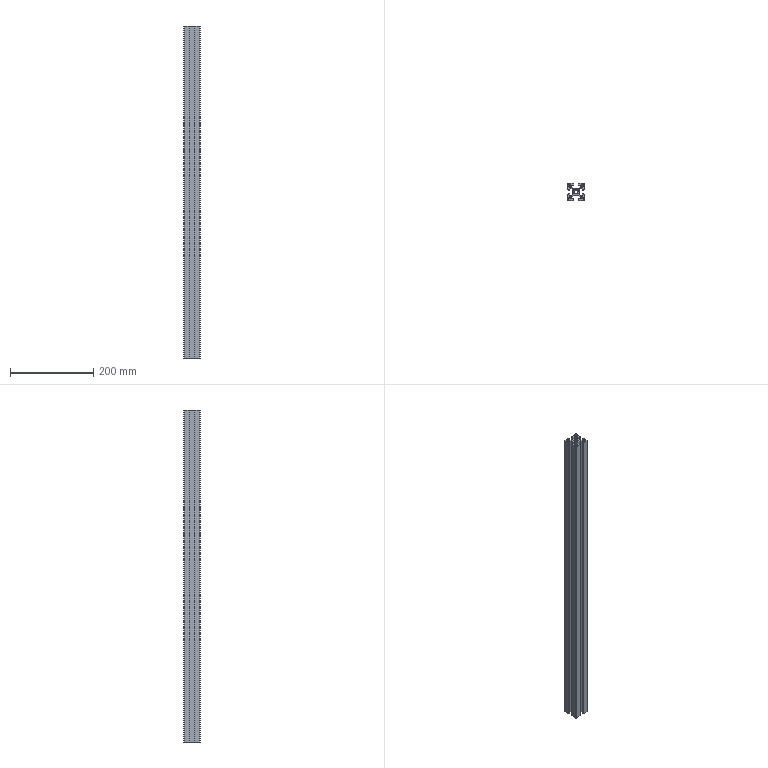Part | SolidWorks | features BaseBody 1 | 1 solid | 125 faces | box 40 x 40 x 800 mm | volume 561173 mm3 | plane 74 | cylinder 51 | commonest cylinder face diameters 2 x24 1.5 x10 5 x8 10.2 x5 4 x4